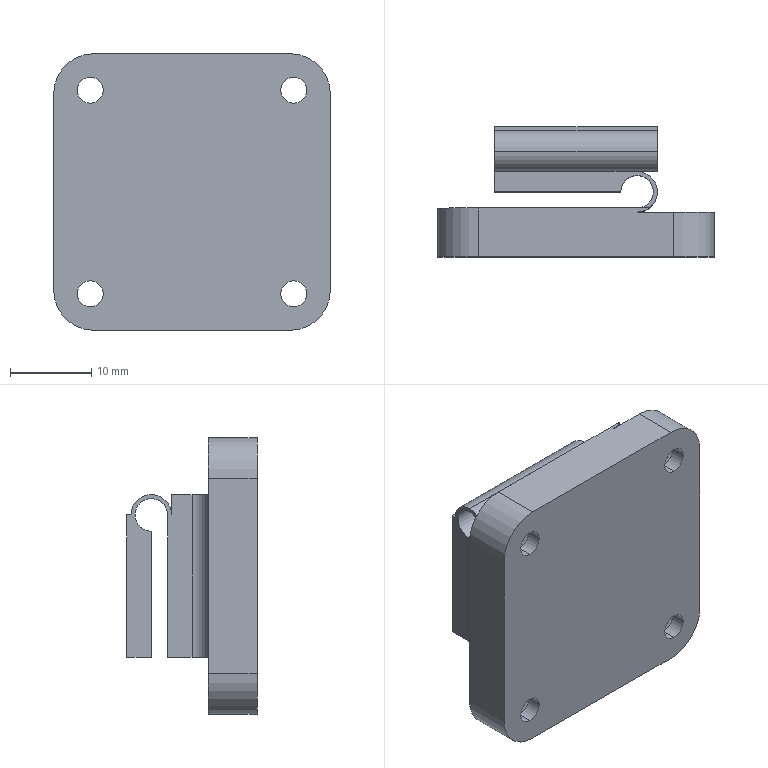Part | SolidWorks | features ICE 9, Extrusion 1, Fillet 1 | 1 solid | 62 faces | box 34 x 16 x 34 mm | volume 8130 mm3 | cylinder 38 | plane 24 | commonest cylinder face diameters 3.2 x8 6.1 x8 3.1 x4 4 x4 5 x4 10 x4